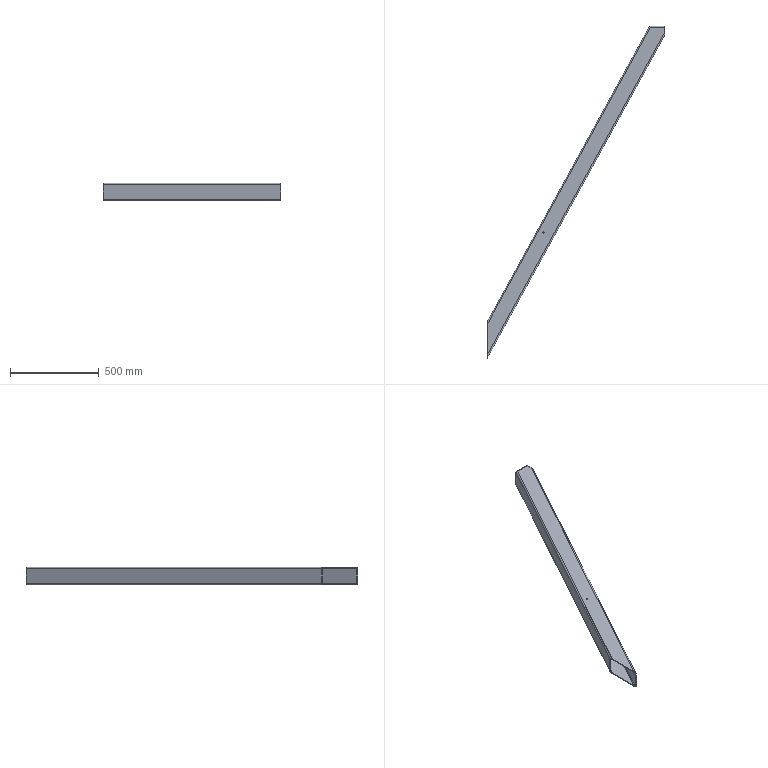Part | SolidWorks | features Fillet 2, Extrusion 1, HoleWzd 1, Shell 1 | 1 solid | 26 faces | box 1000 x 1874 x 100 mm | volume 3026106 mm3 | cylinder 14 | plane 12 | commonest cylinder face diameters 8.4 x6 16.4 x6 6.8 x2
STEP:
#1=CARTESIAN_POINT('',(312.6,708.43,96.));
#2=VERTEX_POINT('',#1);
#3=CARTESIAN_POINT('',(319.4,708.43,96.));
#4=VERTEX_POINT('',#3);
#5=CARTESIAN_POINT('',(316.,708.43,96.));
#6=DIRECTION('',(0.,0.,1.));
#7=DIRECTION('',(1.,0.,0.));
#8=AXIS2_PLACEMENT_3D('',#5,#6,#7);
#9=CIRCLE('',#8,3.4);
#10=EDGE_CURVE('',#2,#4,#9,.T.);
#11=ORIENTED_EDGE('',*,*,#10,.F.);
#12=CARTESIAN_POINT('',(312.6,708.43,100.));
#13=VERTEX_POINT('',#12);
#14=CARTESIAN_POINT('',(312.6,708.43,100.));
#15=DIRECTION('',(0.,0.,1.));
#16=VECTOR('',#15,1000.);
#17=LINE('',#14,#16);
#18=EDGE_CURVE('',#2,#13,#17,.T.);
#19=ORIENTED_EDGE('',*,*,#18,.T.);
#20=CARTESIAN_POINT('',(319.4,708.43,100.));
#21=VERTEX_POINT('',#20);
#22=CARTESIAN_POINT('',(316.,708.43,100.));
#23=DIRECTION('',(0.,0.,1.));
#24=DIRECTION('',(1.,0.,0.));
#25=AXIS2_PLACEMENT_3D('',#22,#23,#24);
#26=CIRCLE('',#25,3.4);
#27=EDGE_CURVE('',#13,#21,#26,.T.);
#28=ORIENTED_EDGE('',*,*,#27,.T.);
#29=CARTESIAN_POINT('',(319.4,708.43,100.));
#30=DIRECTION('',(0.,0.,1.));
#31=VECTOR('',#30,1000.);
#32=LINE('',#29,#31);
#33=EDGE_CURVE('',#4,#21,#32,.T.);
#34=ORIENTED_EDGE('',*,*,#33,.F.);
#35=EDGE_LOOP('',(#11,#19,#28,#34));
#36=FACE_OUTER_BOUND('',#35,.T.);
#37=CARTESIAN_POINT('',(316.,708.43,100.));
#38=DIRECTION('',(0.,0.,1.));
#39=DIRECTION('',(1.,0.,0.));
#40=AXIS2_PLACEMENT_3D('',#37,#38,#39);
#41=CYLINDRICAL_SURFACE('',#40,3.4);
#42=ADVANCED_FACE('',(#36),#41,.F.);
#43=CARTESIAN_POINT('',(1000.,1820.433,91.8));
#44=VERTEX_POINT('',#43);
#45=CARTESIAN_POINT('',(1000.,1820.433,8.2));
#46=VERTEX_POINT('',#45);
#47=CARTESIAN_POINT('',(1000.,1820.433,100.));
#48=DIRECTION('',(0.,0.,-1.));
#49=VECTOR('',#48,1000.);
#50=LINE('',#47,#49);
#51=EDGE_CURVE('',#44,#46,#50,.T.);
#52=ORIENTED_EDGE('',*,*,#51,.T.);
#53=CARTESIAN_POINT('',(1000.,1837.465,0.));
#54=VERTEX_POINT('',#53);
#55=CARTESIAN_POINT('',(1000.,1820.433,8.2));
#56=CARTESIAN_POINT('',(1000.,1820.433,3.397));
#57=CARTESIAN_POINT('',(1000.,1827.488,0.));
#58=CARTESIAN_POINT('',(1000.,1837.465,0.));
#59=(BOUNDED_CURVE()B_SPLINE_CURVE(3,(#55,#56,#57,#58),.UNSPECIFIED.,.F.,.F.)B_SPLINE_CURVE_WITH_KNOTS((4,4),(3.142,4.712),.UNSPECIFIED.)CURVE()GEOMETRIC_REPRESENTATION_ITEM()RATIONAL_B_SPLINE_CURVE((1.,0.8047,0.8047,1.))REPRESENTATION_ITEM(''));
#60=EDGE_CURVE('',#46,#54,#59,.T.);
#61=ORIENTED_EDGE('',*,*,#60,.T.);
#62=CARTESIAN_POINT('',(1000.,1866.233,0.));
#63=VERTEX_POINT('',#62);
#64=CARTESIAN_POINT('',(1000.,1874.433,0.));
#65=DIRECTION('',(0.,-1.,0.));
#66=VECTOR('',#65,1000.);
#67=LINE('',#64,#66);
#68=EDGE_CURVE('',#63,#54,#67,.T.);
#69=ORIENTED_EDGE('',*,*,#68,.F.);
#70=CARTESIAN_POINT('',(1000.,1874.433,8.2));
#71=VERTEX_POINT('',#70);
#72=CARTESIAN_POINT('',(1000.,1866.233,8.2));
#73=DIRECTION('',(1.,0.,0.));
#74=DIRECTION('',(0.,1.,0.));
#75=AXIS2_PLACEMENT_3D('',#72,#73,#74);
#76=CIRCLE('',#75,8.2);
#77=EDGE_CURVE('',#63,#71,#76,.T.);
#78=ORIENTED_EDGE('',*,*,#77,.T.);
#79=CARTESIAN_POINT('',(1000.,1874.433,91.8));
#80=VERTEX_POINT('',#79);
#81=CARTESIAN_POINT('',(1000.,1874.433,100.));
#82=DIRECTION('',(0.,0.,-1.));
#83=VECTOR('',#82,1000.);
#84=LINE('',#81,#83);
#85=EDGE_CURVE('',#80,#71,#84,.T.);
#86=ORIENTED_EDGE('',*,*,#85,.F.);
#87=CARTESIAN_POINT('',(1000.,1866.233,100.));
#88=VERTEX_POINT('',#87);
#89=CARTESIAN_POINT('',(1000.,1866.233,91.8));
#90=DIRECTION('',(1.,0.,0.));
#91=DIRECTION('',(0.,1.,0.));
#92=AXIS2_PLACEMENT_3D('',#89,#90,#91);
#93=CIRCLE('',#92,8.2);
#94=EDGE_CURVE('',#80,#88,#93,.T.);
#95=ORIENTED_EDGE('',*,*,#94,.T.);
#96=CARTESIAN_POINT('',(1000.,1837.465,100.));
#97=VERTEX_POINT('',#96);
#98=CARTESIAN_POINT('',(1000.,1874.433,100.));
#99=DIRECTION('',(0.,-1.,0.));
#100=VECTOR('',#99,1000.);
#101=LINE('',#98,#100);
#102=EDGE_CURVE('',#88,#97,#101,.T.);
#103=ORIENTED_EDGE('',*,*,#102,.T.);
#104=CARTESIAN_POINT('',(1000.,1837.465,100.));
#105=CARTESIAN_POINT('',(1000.,1827.488,100.));
#106=CARTESIAN_POINT('',(1000.,1820.433,96.603));
#107=CARTESIAN_POINT('',(1000.,1820.433,91.8));
#108=(BOUNDED_CURVE()B_SPLINE_CURVE(3,(#104,#105,#106,#107),.UNSPECIFIED.,.F.,.F.)B_SPLINE_CURVE_WITH_KNOTS((4,4),(4.712,6.283),.UNSPECIFIED.)CURVE()GEOMETRIC_REPRESENTATION_ITEM()RATIONAL_B_SPLINE_CURVE((1.,0.8047,0.8047,1.))REPRESENTATION_ITEM(''));
#109=EDGE_CURVE('',#97,#44,#108,.T.);
#110=ORIENTED_EDGE('',*,*,#109,.T.);
#111=EDGE_LOOP('',(#52,#61,#69,#78,#86,#95,#103,#110));
#112=FACE_OUTER_BOUND('',#111,.T.);
#113=CARTESIAN_POINT('',(1000.,1866.233,96.));
#114=VERTEX_POINT('',#113);
#115=CARTESIAN_POINT('',(1000.,1837.465,96.));
#116=VERTEX_POINT('',#115);
#117=CARTESIAN_POINT('',(1000.,1874.433,96.));
#118=DIRECTION('',(0.,-1.,0.));
#119=VECTOR('',#118,1000.);
#120=LINE('',#117,#119);
#121=EDGE_CURVE('',#114,#116,#120,.T.);
#122=ORIENTED_EDGE('',*,*,#121,.F.);
#123=CARTESIAN_POINT('',(1000.,1870.433,91.8));
#124=VERTEX_POINT('',#123);
#125=CARTESIAN_POINT('',(1000.,1866.233,91.8));
#126=DIRECTION('',(-1.,0.,0.));
#127=DIRECTION('',(0.,1.,0.));
#128=AXIS2_PLACEMENT_3D('',#125,#126,#127);
#129=CIRCLE('',#128,4.2);
#130=EDGE_CURVE('',#114,#124,#129,.T.);
#131=ORIENTED_EDGE('',*,*,#130,.T.);
#132=CARTESIAN_POINT('',(1000.,1870.433,8.2));
#133=VERTEX_POINT('',#132);
#134=CARTESIAN_POINT('',(1000.,1870.433,100.));
#135=DIRECTION('',(0.,0.,-1.));
#136=VECTOR('',#135,1000.);
#137=LINE('',#134,#136);
#138=EDGE_CURVE('',#124,#133,#137,.T.);
#139=ORIENTED_EDGE('',*,*,#138,.T.);
#140=CARTESIAN_POINT('',(1000.,1866.233,4.));
#141=VERTEX_POINT('',#140);
#142=CARTESIAN_POINT('',(1000.,1866.233,8.2));
#143=DIRECTION('',(-1.,0.,0.));
#144=DIRECTION('',(0.,1.,0.));
#145=AXIS2_PLACEMENT_3D('',#142,#143,#144);
#146=CIRCLE('',#145,4.2);
#147=EDGE_CURVE('',#133,#141,#146,.T.);
#148=ORIENTED_EDGE('',*,*,#147,.T.);
#149=CARTESIAN_POINT('',(1000.,1837.465,4.));
#150=VERTEX_POINT('',#149);
#151=CARTESIAN_POINT('',(1000.,1874.433,4.));
#152=DIRECTION('',(0.,-1.,0.));
#153=VECTOR('',#152,1000.);
#154=LINE('',#151,#153);
#155=EDGE_CURVE('',#141,#150,#154,.T.);
#156=ORIENTED_EDGE('',*,*,#155,.T.);
#157=CARTESIAN_POINT('',(1000.,1828.741,8.2));
#158=VERTEX_POINT('',#157);
#159=CARTESIAN_POINT('',(1000.,1837.465,4.));
#160=CARTESIAN_POINT('',(1000.,1832.355,4.));
#161=CARTESIAN_POINT('',(1000.,1828.741,5.74));
#162=CARTESIAN_POINT('',(1000.,1828.741,8.2));
#163=(BOUNDED_CURVE()B_SPLINE_CURVE(3,(#159,#160,#161,#162),.UNSPECIFIED.,.F.,.F.)B_SPLINE_CURVE_WITH_KNOTS((4,4),(4.712,6.283),.UNSPECIFIED.)CURVE()GEOMETRIC_REPRESENTATION_ITEM()RATIONAL_B_SPLINE_CURVE((1.,0.8047,0.8047,1.))REPRESENTATION_ITEM(''));
#164=EDGE_CURVE('',#150,#158,#163,.T.);
#165=ORIENTED_EDGE('',*,*,#164,.T.);
#166=CARTESIAN_POINT('',(1000.,1828.741,91.8));
#167=VERTEX_POINT('',#166);
#168=CARTESIAN_POINT('',(1000.,1828.741,100.));
#169=DIRECTION('',(0.,0.,-1.));
#170=VECTOR('',#169,1000.);
#171=LINE('',#168,#170);
#172=EDGE_CURVE('',#167,#158,#171,.T.);
#173=ORIENTED_EDGE('',*,*,#172,.F.);
#174=CARTESIAN_POINT('',(1000.,1828.741,91.8));
#175=CARTESIAN_POINT('',(1000.,1828.741,94.26));
#176=CARTESIAN_POINT('',(1000.,1832.355,96.));
#177=CARTESIAN_POINT('',(1000.,1837.465,96.));
#178=(BOUNDED_CURVE()B_SPLINE_CURVE(3,(#174,#175,#176,#177),.UNSPECIFIED.,.F.,.F.)B_SPLINE_CURVE_WITH_KNOTS((4,4),(3.142,4.712),.UNSPECIFIED.)CURVE()GEOMETRIC_REPRESENTATION_ITEM()RATIONAL_B_SPLINE_CURVE((1.,0.8047,0.8047,1.))REPRESENTATION_ITEM(''));
#179=EDGE_CURVE('',#167,#116,#178,.T.);
#180=ORIENTED_EDGE('',*,*,#179,.T.);
#181=EDGE_LOOP('',(#122,#131,#139,#148,#156,#165,#173,#180));
#182=FACE_BOUND('',#181,.T.);
#183=CARTESIAN_POINT('',(1000.,1874.433,100.));
#184=DIRECTION('',(1.,0.,0.));
#185=DIRECTION('',(0.,1.,0.));
#186=AXIS2_PLACEMENT_3D('',#183,#184,#185);
#187=PLANE('',#186);
#188=ADVANCED_FACE('',(#112,#182),#187,.T.);
#189=CARTESIAN_POINT('',(0.,17.031,0.));
#190=VERTEX_POINT('',#189);
#191=CARTESIAN_POINT('',(0.,191.705,0.));
#192=VERTEX_POINT('',#191);
#193=CARTESIAN_POINT('',(0.,0.,0.));
#194=DIRECTION('',(0.,1.,0.));
#195=VECTOR('',#194,1000.);
#196=LINE('',#193,#195);
#197=EDGE_CURVE('',#190,#192,#196,.T.);
#198=ORIENTED_EDGE('',*,*,#197,.F.);
#199=CARTESIAN_POINT('',(0.,0.,8.2));
#200=VERTEX_POINT('',#199);
#201=CARTESIAN_POINT('',(0.,17.031,0.));
#202=CARTESIAN_POINT('',(0.,7.055,0.));
#203=CARTESIAN_POINT('',(0.,0.,3.397));
#204=CARTESIAN_POINT('',(0.,0.,8.2));
#205=(BOUNDED_CURVE()B_SPLINE_CURVE(3,(#201,#202,#203,#204),.UNSPECIFIED.,.F.,.F.)B_SPLINE_CURVE_WITH_KNOTS((4,4),(1.571,3.142),.UNSPECIFIED.)CURVE()GEOMETRIC_REPRESENTATION_ITEM()RATIONAL_B_SPLINE_CURVE((1.,0.8047,0.8047,1.))REPRESENTATION_ITEM(''));
#206=EDGE_CURVE('',#190,#200,#205,.T.);
#207=ORIENTED_EDGE('',*,*,#206,.T.);
#208=CARTESIAN_POINT('',(0.,0.,91.8));
#209=VERTEX_POINT('',#208);
#210=CARTESIAN_POINT('',(0.,0.,100.));
#211=DIRECTION('',(0.,0.,-1.));
#212=VECTOR('',#211,1000.);
#213=LINE('',#210,#212);
#214=EDGE_CURVE('',#209,#200,#213,.T.);
#215=ORIENTED_EDGE('',*,*,#214,.F.);
#216=CARTESIAN_POINT('',(0.,17.031,100.));
#217=VERTEX_POINT('',#216);
#218=CARTESIAN_POINT('',(0.,0.,91.8));
#219=CARTESIAN_POINT('',(0.,0.,96.603));
#220=CARTESIAN_POINT('',(0.,7.055,100.));
#221=CARTESIAN_POINT('',(0.,17.031,100.));
#222=(BOUNDED_CURVE()B_SPLINE_CURVE(3,(#218,#219,#220,#221),.UNSPECIFIED.,.F.,.F.)B_SPLINE_CURVE_WITH_KNOTS((4,4),(0.,1.571),.UNSPECIFIED.)CURVE()GEOMETRIC_REPRESENTATION_ITEM()RATIONAL_B_SPLINE_CURVE((1.,0.8047,0.8047,1.))REPRESENTATION_ITEM(''));
#223=EDGE_CURVE('',#209,#217,#222,.T.);
#224=ORIENTED_EDGE('',*,*,#223,.T.);
#225=CARTESIAN_POINT('',(0.,191.705,100.));
#226=VERTEX_POINT('',#225);
#227=CARTESIAN_POINT('',(0.,0.,100.));
#228=DIRECTION('',(0.,1.,0.));
#229=VECTOR('',#228,1000.);
#230=LINE('',#227,#229);
#231=EDGE_CURVE('',#217,#226,#230,.T.);
#232=ORIENTED_EDGE('',*,*,#231,.T.);
#233=CARTESIAN_POINT('',(0.,208.737,91.8));
#234=VERTEX_POINT('',#233);
#235=CARTESIAN_POINT('',(0.,191.705,100.));
#236=CARTESIAN_POINT('',(0.,201.682,100.));
#237=CARTESIAN_POINT('',(0.,208.737,96.603));
#238=CARTESIAN_POINT('',(0.,208.737,91.8));
#239=(BOUNDED_CURVE()B_SPLINE_CURVE(3,(#235,#236,#237,#238),.UNSPECIFIED.,.F.,.T.)B_SPLINE_CURVE_WITH_KNOTS((4,4),(4.712,6.283),.UNSPECIFIED.)CURVE()GEOMETRIC_REPRESENTATION_ITEM()RATIONAL_B_SPLINE_CURVE((1.,0.8047,0.8047,1.))REPRESENTATION_ITEM(''));
#240=EDGE_CURVE('',#226,#234,#239,.T.);
#241=ORIENTED_EDGE('',*,*,#240,.T.);
#242=CARTESIAN_POINT('',(0.,208.737,8.2));
#243=VERTEX_POINT('',#242);
#244=CARTESIAN_POINT('',(0.,208.737,100.));
#245=DIRECTION('',(0.,0.,-1.));
#246=VECTOR('',#245,1000.);
#247=LINE('',#244,#246);
#248=EDGE_CURVE('',#234,#243,#247,.T.);
#249=ORIENTED_EDGE('',*,*,#248,.T.);
#250=CARTESIAN_POINT('',(0.,208.737,8.2));
#251=CARTESIAN_POINT('',(0.,208.737,3.397));
#252=CARTESIAN_POINT('',(0.,201.682,0.));
#253=CARTESIAN_POINT('',(0.,191.705,0.));
#254=(BOUNDED_CURVE()B_SPLINE_CURVE(3,(#250,#251,#252,#253),.UNSPECIFIED.,.F.,.F.)B_SPLINE_CURVE_WITH_KNOTS((4,4),(3.142,4.712),.UNSPECIFIED.)CURVE()GEOMETRIC_REPRESENTATION_ITEM()RATIONAL_B_SPLINE_CURVE((1.,0.8047,0.8047,1.))REPRESENTATION_ITEM(''));
#255=EDGE_CURVE('',#243,#192,#254,.T.);
#256=ORIENTED_EDGE('',*,*,#255,.T.);
#257=EDGE_LOOP('',(#198,#207,#215,#224,#232,#241,#249,#256));
#258=FACE_OUTER_BOUND('',#257,.T.);
#259=CARTESIAN_POINT('',(0.,17.031,96.));
#260=VERTEX_POINT('',#259);
#261=CARTESIAN_POINT('',(0.,191.705,96.));
#262=VERTEX_POINT('',#261);
#263=CARTESIAN_POINT('',(0.,0.,96.));
#264=DIRECTION('',(0.,1.,0.));
#265=VECTOR('',#264,1000.);
#266=LINE('',#263,#265);
#267=EDGE_CURVE('',#260,#262,#266,.T.);
#268=ORIENTED_EDGE('',*,*,#267,.F.);
#269=CARTESIAN_POINT('',(0.,8.308,91.8));
#270=VERTEX_POINT('',#269);
#271=CARTESIAN_POINT('',(0.,17.031,96.));
#272=CARTESIAN_POINT('',(0.,11.921,96.));
#273=CARTESIAN_POINT('',(0.,8.308,94.26));
#274=CARTESIAN_POINT('',(0.,8.308,91.8));
#275=(BOUNDED_CURVE()B_SPLINE_CURVE(3,(#271,#272,#273,#274),.UNSPECIFIED.,.F.,.F.)B_SPLINE_CURVE_WITH_KNOTS((4,4),(1.571,3.142),.UNSPECIFIED.)CURVE()GEOMETRIC_REPRESENTATION_ITEM()RATIONAL_B_SPLINE_CURVE((1.,0.8047,0.8047,1.))REPRESENTATION_ITEM(''));
#276=EDGE_CURVE('',#260,#270,#275,.T.);
#277=ORIENTED_EDGE('',*,*,#276,.T.);
#278=CARTESIAN_POINT('',(0.,8.308,8.2));
#279=VERTEX_POINT('',#278);
#280=CARTESIAN_POINT('',(0.,8.308,100.));
#281=DIRECTION('',(0.,0.,-1.));
#282=VECTOR('',#281,1000.);
#283=LINE('',#280,#282);
#284=EDGE_CURVE('',#270,#279,#283,.T.);
#285=ORIENTED_EDGE('',*,*,#284,.T.);
#286=CARTESIAN_POINT('',(0.,17.031,4.));
#287=VERTEX_POINT('',#286);
#288=CARTESIAN_POINT('',(0.,8.308,8.2));
#289=CARTESIAN_POINT('',(0.,8.308,5.74));
#290=CARTESIAN_POINT('',(0.,11.921,4.));
#291=CARTESIAN_POINT('',(0.,17.031,4.));
#292=(BOUNDED_CURVE()B_SPLINE_CURVE(3,(#288,#289,#290,#291),.UNSPECIFIED.,.F.,.F.)B_SPLINE_CURVE_WITH_KNOTS((4,4),(0.,1.571),.UNSPECIFIED.)CURVE()GEOMETRIC_REPRESENTATION_ITEM()RATIONAL_B_SPLINE_CURVE((1.,0.8047,0.8047,1.))REPRESENTATION_ITEM(''));
#293=EDGE_CURVE('',#279,#287,#292,.T.);
#294=ORIENTED_EDGE('',*,*,#293,.T.);
#295=CARTESIAN_POINT('',(0.,191.705,4.));
#296=VERTEX_POINT('',#295);
#297=CARTESIAN_POINT('',(0.,0.,4.));
#298=DIRECTION('',(0.,1.,0.));
#299=VECTOR('',#298,1000.);
#300=LINE('',#297,#299);
#301=EDGE_CURVE('',#287,#296,#300,.T.);
#302=ORIENTED_EDGE('',*,*,#301,.T.);
#303=CARTESIAN_POINT('',(0.,200.429,8.2));
#304=VERTEX_POINT('',#303);
#305=CARTESIAN_POINT('',(0.,191.705,4.));
#306=CARTESIAN_POINT('',(0.,196.815,4.));
#307=CARTESIAN_POINT('',(0.,200.429,5.74));
#308=CARTESIAN_POINT('',(0.,200.429,8.2));
#309=(BOUNDED_CURVE()B_SPLINE_CURVE(3,(#305,#306,#307,#308),.UNSPECIFIED.,.F.,.F.)B_SPLINE_CURVE_WITH_KNOTS((4,4),(4.712,6.283),.UNSPECIFIED.)CURVE()GEOMETRIC_REPRESENTATION_ITEM()RATIONAL_B_SPLINE_CURVE((1.,0.8047,0.8047,1.))REPRESENTATION_ITEM(''));
#310=EDGE_CURVE('',#296,#304,#309,.T.);
#311=ORIENTED_EDGE('',*,*,#310,.T.);
#312=CARTESIAN_POINT('',(0.,200.429,91.8));
#313=VERTEX_POINT('',#312);
#314=CARTESIAN_POINT('',(0.,200.429,100.));
#315=DIRECTION('',(0.,0.,-1.));
#316=VECTOR('',#315,1000.);
#317=LINE('',#314,#316);
#318=EDGE_CURVE('',#313,#304,#317,.T.);
#319=ORIENTED_EDGE('',*,*,#318,.F.);
#320=CARTESIAN_POINT('',(0.,200.429,91.8));
#321=CARTESIAN_POINT('',(0.,200.429,94.26));
#322=CARTESIAN_POINT('',(0.,196.815,96.));
#323=CARTESIAN_POINT('',(0.,191.705,96.));
#324=(BOUNDED_CURVE()B_SPLINE_CURVE(3,(#320,#321,#322,#323),.UNSPECIFIED.,.F.,.T.)B_SPLINE_CURVE_WITH_KNOTS((4,4),(3.142,4.712),.UNSPECIFIED.)CURVE()GEOMETRIC_REPRESENTATION_ITEM()RATIONAL_B_SPLINE_CURVE((1.,0.8047,0.8047,1.))REPRESENTATION_ITEM(''));
#325=EDGE_CURVE('',#313,#262,#324,.T.);
#326=ORIENTED_EDGE('',*,*,#325,.T.);
#327=EDGE_LOOP('',(#268,#277,#285,#294,#302,#311,#319,#326));
#328=FACE_BOUND('',#327,.T.);
#329=CARTESIAN_POINT('',(0.,0.,100.));
#330=DIRECTION('',(-1.,0.,0.));
#331=DIRECTION('',(0.,-1.,0.));
#332=AXIS2_PLACEMENT_3D('',#329,#330,#331);
#333=PLANE('',#332);
#334=ADVANCED_FACE('',(#258,#328),#333,.T.);
#335=ORIENTED_EDGE('',*,*,#85,.T.);
#336=CARTESIAN_POINT('',(915.,1874.433,8.2));
#337=VERTEX_POINT('',#336);
#338=CARTESIAN_POINT('',(915.,1874.433,8.2));
#339=DIRECTION('',(-1.,0.,0.));
#340=VECTOR('',#339,1000.);
#341=LINE('',#338,#340);
#342=EDGE_CURVE('',#71,#337,#341,.T.);
#343=ORIENTED_EDGE('',*,*,#342,.T.);
#344=CARTESIAN_POINT('',(915.,1874.433,91.8));
#345=VERTEX_POINT('',#344);
#346=CARTESIAN_POINT('',(915.,1874.433,100.));
#347=DIRECTION('',(0.,0.,-1.));
#348=VECTOR('',#347,1000.);
#349=LINE('',#346,#348);
#350=EDGE_CURVE('',#345,#337,#349,.T.);
#351=ORIENTED_EDGE('',*,*,#350,.F.);
#352=CARTESIAN_POINT('',(915.,1874.433,91.8));
#353=DIRECTION('',(1.,0.,0.));
#354=VECTOR('',#353,1000.);
#355=LINE('',#352,#354);
#356=EDGE_CURVE('',#345,#80,#355,.T.);
#357=ORIENTED_EDGE('',*,*,#356,.T.);
#358=EDGE_LOOP('',(#335,#343,#351,#357));
#359=FACE_OUTER_BOUND('',#358,.T.);
#360=CARTESIAN_POINT('',(915.,1874.433,100.));
#361=DIRECTION('',(0.,1.,0.));
#362=DIRECTION('',(-1.,0.,0.));
#363=AXIS2_PLACEMENT_3D('',#360,#361,#362);
#364=PLANE('',#363);
#365=ADVANCED_FACE('',(#359),#364,.T.);
#366=ORIENTED_EDGE('',*,*,#350,.T.);
#367=CARTESIAN_POINT('',(0.,208.737,8.2));
#368=DIRECTION('',(-0.4815,-0.8765,0.));
#369=VECTOR('',#368,1000.);
#370=LINE('',#367,#369);
#371=EDGE_CURVE('',#337,#243,#370,.T.);
#372=ORIENTED_EDGE('',*,*,#371,.T.);
#373=ORIENTED_EDGE('',*,*,#248,.F.);
#374=CARTESIAN_POINT('',(0.,208.737,91.8));
#375=DIRECTION('',(0.4815,0.8765,0.));
#376=VECTOR('',#375,1000.);
#377=LINE('',#374,#376);
#378=EDGE_CURVE('',#234,#345,#377,.T.);
#379=ORIENTED_EDGE('',*,*,#378,.T.);
#380=EDGE_LOOP('',(#366,#372,#373,#379));
#381=FACE_OUTER_BOUND('',#380,.T.);
#382=CARTESIAN_POINT('',(0.,208.737,100.));
#383=DIRECTION('',(-0.8765,0.4815,0.));
#384=DIRECTION('',(-0.4815,-0.8765,0.));
#385=AXIS2_PLACEMENT_3D('',#382,#383,#384);
#386=PLANE('',#385);
#387=ADVANCED_FACE('',(#381),#386,.T.);
#388=ORIENTED_EDGE('',*,*,#214,.T.);
#389=CARTESIAN_POINT('',(1000.,1820.433,8.2));
#390=DIRECTION('',(0.4815,0.8765,0.));
#391=VECTOR('',#390,1000.);
#392=LINE('',#389,#391);
#393=EDGE_CURVE('',#200,#46,#392,.T.);
#394=ORIENTED_EDGE('',*,*,#393,.T.);
#395=ORIENTED_EDGE('',*,*,#51,.F.);
#396=CARTESIAN_POINT('',(1000.,1820.433,91.8));
#397=DIRECTION('',(-0.4815,-0.8765,0.));
#398=VECTOR('',#397,1000.);
#399=LINE('',#396,#398);
#400=EDGE_CURVE('',#44,#209,#399,.T.);
#401=ORIENTED_EDGE('',*,*,#400,.T.);
#402=EDGE_LOOP('',(#388,#394,#395,#401));
#403=FACE_OUTER_BOUND('',#402,.T.);
#404=CARTESIAN_POINT('',(1000.,1820.433,100.));
#405=DIRECTION('',(0.8765,-0.4815,0.));
#406=DIRECTION('',(0.4815,0.8765,0.));
#407=AXIS2_PLACEMENT_3D('',#404,#405,#406);
#408=PLANE('',#407);
#409=ADVANCED_FACE('',(#403),#408,.T.);
#410=CARTESIAN_POINT('',(316.,708.43,100.));
#411=DIRECTION('',(0.,0.,1.));
#412=DIRECTION('',(1.,0.,0.));
#413=AXIS2_PLACEMENT_3D('',#410,#411,#412);
#414=CIRCLE('',#413,3.4);
#415=EDGE_CURVE('',#21,#13,#414,.T.);
#416=ORIENTED_EDGE('',*,*,#415,.F.);
#417=ORIENTED_EDGE('',*,*,#27,.F.);
#418=EDGE_LOOP('',(#416,#417));
#419=FACE_BOUND('',#418,.T.);
#420=ORIENTED_EDGE('',*,*,#231,.F.);
#421=CARTESIAN_POINT('',(-7.187,3.948,100.));
#422=DIRECTION('',(0.4815,0.8765,0.));
#423=VECTOR('',#422,1000.);
#424=LINE('',#421,#423);
#425=EDGE_CURVE('',#217,#97,#424,.T.);
#426=ORIENTED_EDGE('',*,*,#425,.T.);
#427=ORIENTED_EDGE('',*,*,#102,.F.);
#428=CARTESIAN_POINT('',(919.851,1866.233,100.));
#429=VERTEX_POINT('',#428);
#430=CARTESIAN_POINT('',(0.,1866.233,100.));
#431=DIRECTION('',(-1.,0.,0.));
#432=VECTOR('',#431,1000.);
#433=LINE('',#430,#432);
#434=EDGE_CURVE('',#88,#429,#433,.T.);
#435=ORIENTED_EDGE('',*,*,#434,.T.);
#436=CARTESIAN_POINT('',(-80.897,44.438,100.));
#437=DIRECTION('',(-0.4815,-0.8765,0.));
#438=VECTOR('',#437,1000.);
#439=LINE('',#436,#438);
#440=EDGE_CURVE('',#429,#226,#439,.T.);
#441=ORIENTED_EDGE('',*,*,#440,.T.);
#442=EDGE_LOOP('',(#420,#426,#427,#435,#441));
#443=FACE_OUTER_BOUND('',#442,.T.);
#444=CARTESIAN_POINT('',(0.,0.,100.));
#445=DIRECTION('',(0.,0.,1.));
#446=DIRECTION('',(1.,0.,0.));
#447=AXIS2_PLACEMENT_3D('',#444,#445,#446);
#448=PLANE('',#447);
#449=ADVANCED_FACE('',(#419,#443),#448,.T.);
#450=ORIENTED_EDGE('',*,*,#68,.T.);
#451=CARTESIAN_POINT('',(-7.187,3.948,0.));
#452=DIRECTION('',(-0.4815,-0.8765,0.));
#453=VECTOR('',#452,1000.);
#454=LINE('',#451,#453);
#455=EDGE_CURVE('',#54,#190,#454,.T.);
#456=ORIENTED_EDGE('',*,*,#455,.T.);
#457=ORIENTED_EDGE('',*,*,#197,.T.);
#458=CARTESIAN_POINT('',(919.851,1866.233,0.));
#459=VERTEX_POINT('',#458);
#460=CARTESIAN_POINT('',(922.187,1870.485,0.));
#461=DIRECTION('',(0.4815,0.8765,0.));
#462=VECTOR('',#461,1000.);
#463=LINE('',#460,#462);
#464=EDGE_CURVE('',#192,#459,#463,.T.);
#465=ORIENTED_EDGE('',*,*,#464,.T.);
#466=CARTESIAN_POINT('',(1000.,1866.233,0.));
#467=DIRECTION('',(1.,0.,0.));
#468=VECTOR('',#467,1000.);
#469=LINE('',#466,#468);
#470=EDGE_CURVE('',#459,#63,#469,.T.);
#471=ORIENTED_EDGE('',*,*,#470,.T.);
#472=EDGE_LOOP('',(#450,#456,#457,#465,#471));
#473=FACE_OUTER_BOUND('',#472,.T.);
#474=CARTESIAN_POINT('',(0.,0.,0.));
#475=DIRECTION('',(0.,0.,1.));
#476=DIRECTION('',(1.,0.,0.));
#477=AXIS2_PLACEMENT_3D('',#474,#475,#476);
#478=PLANE('',#477);
#479=ADVANCED_FACE('',(#473),#478,.F.);
#480=ORIENTED_EDGE('',*,*,#138,.F.);
#481=CARTESIAN_POINT('',(917.366,1870.433,91.8));
#482=VERTEX_POINT('',#481);
#483=CARTESIAN_POINT('',(917.366,1870.433,91.8));
#484=DIRECTION('',(-1.,0.,0.));
#485=VECTOR('',#484,1000.);
#486=LINE('',#483,#485);
#487=EDGE_CURVE('',#124,#482,#486,.T.);
#488=ORIENTED_EDGE('',*,*,#487,.T.);
#489=CARTESIAN_POINT('',(917.366,1870.433,8.2));
#490=VERTEX_POINT('',#489);
#491=CARTESIAN_POINT('',(917.366,1870.433,100.));
#492=DIRECTION('',(0.,0.,-1.));
#493=VECTOR('',#492,1000.);
#494=LINE('',#491,#493);
#495=EDGE_CURVE('',#482,#490,#494,.T.);
#496=ORIENTED_EDGE('',*,*,#495,.T.);
#497=CARTESIAN_POINT('',(915.,1870.433,8.2));
#498=DIRECTION('',(1.,0.,0.));
#499=VECTOR('',#498,1000.);
#500=LINE('',#497,#499);
#501=EDGE_CURVE('',#490,#133,#500,.T.);
#502=ORIENTED_EDGE('',*,*,#501,.T.);
#503=EDGE_LOOP('',(#480,#488,#496,#502));
#504=FACE_OUTER_BOUND('',#503,.T.);
#505=CARTESIAN_POINT('',(915.,1870.433,100.));
#506=DIRECTION('',(0.,1.,0.));
#507=DIRECTION('',(-1.,0.,0.));
#508=AXIS2_PLACEMENT_3D('',#505,#506,#507);
#509=PLANE('',#508);
#510=ADVANCED_FACE('',(#504),#509,.F.);
#511=ORIENTED_EDGE('',*,*,#318,.T.);
#512=CARTESIAN_POINT('',(3.506,206.811,8.2));
#513=DIRECTION('',(0.4815,0.8765,0.));
#514=VECTOR('',#513,1000.);
#515=LINE('',#512,#514);
#516=EDGE_CURVE('',#304,#490,#515,.T.);
#517=ORIENTED_EDGE('',*,*,#516,.T.);
#518=ORIENTED_EDGE('',*,*,#495,.F.);
#519=CARTESIAN_POINT('',(0.,200.429,91.8));
#520=DIRECTION('',(-0.4815,-0.8765,0.));
#521=VECTOR('',#520,1000.);
#522=LINE('',#519,#521);
#523=EDGE_CURVE('',#482,#313,#522,.T.);
#524=ORIENTED_EDGE('',*,*,#523,.T.);
#525=EDGE_LOOP('',(#511,#517,#518,#524));
#526=FACE_OUTER_BOUND('',#525,.T.);
#527=CARTESIAN_POINT('',(3.506,206.811,100.));
#528=DIRECTION('',(-0.8765,0.4815,0.));
#529=DIRECTION('',(-0.4815,-0.8765,0.));
#530=AXIS2_PLACEMENT_3D('',#527,#528,#529);
#531=PLANE('',#530);
#532=ADVANCED_FACE('',(#526),#531,.F.);
#533=ORIENTED_EDGE('',*,*,#284,.F.);
#534=CARTESIAN_POINT('',(1000.,1828.741,91.8));
#535=DIRECTION('',(0.4815,0.8765,0.));
#536=VECTOR('',#535,1000.);
#537=LINE('',#534,#536);
#538=EDGE_CURVE('',#270,#167,#537,.T.);
#539=ORIENTED_EDGE('',*,*,#538,.T.);
#540=ORIENTED_EDGE('',*,*,#172,.T.);
#541=CARTESIAN_POINT('',(996.494,1822.359,8.2));
#542=DIRECTION('',(-0.4815,-0.8765,0.));
#543=VECTOR('',#542,1000.);
#544=LINE('',#541,#543);
#545=EDGE_CURVE('',#158,#279,#544,.T.);
#546=ORIENTED_EDGE('',*,*,#545,.T.);
#547=EDGE_LOOP('',(#533,#539,#540,#546));
#548=FACE_OUTER_BOUND('',#547,.T.);
#549=CARTESIAN_POINT('',(996.494,1822.359,100.));
#550=DIRECTION('',(0.8765,-0.4815,0.));
#551=DIRECTION('',(0.4815,0.8765,0.));
#552=AXIS2_PLACEMENT_3D('',#549,#550,#551);
#553=PLANE('',#552);
#554=ADVANCED_FACE('',(#548),#553,.F.);
#555=CARTESIAN_POINT('',(316.,708.43,96.));
#556=DIRECTION('',(0.,0.,1.));
#557=DIRECTION('',(1.,0.,0.));
#558=AXIS2_PLACEMENT_3D('',#555,#556,#557);
#559=CIRCLE('',#558,3.4);
#560=EDGE_CURVE('',#4,#2,#559,.T.);
#561=ORIENTED_EDGE('',*,*,#560,.T.);
#562=ORIENTED_EDGE('',*,*,#10,.T.);
#563=EDGE_LOOP('',(#561,#562));
#564=FACE_BOUND('',#563,.T.);
#565=ORIENTED_EDGE('',*,*,#121,.T.);
#566=CARTESIAN_POINT('',(-3.681,10.33,96.));
#567=DIRECTION('',(-0.4815,-0.8765,0.));
#568=VECTOR('',#567,1000.);
#569=LINE('',#566,#568);
#570=EDGE_CURVE('',#116,#260,#569,.T.);
#571=ORIENTED_EDGE('',*,*,#570,.T.);
#572=ORIENTED_EDGE('',*,*,#267,.T.);
#573=CARTESIAN_POINT('',(919.851,1866.233,96.));
#574=VERTEX_POINT('',#573);
#575=CARTESIAN_POINT('',(921.048,1868.411,96.));
#576=DIRECTION('',(0.4815,0.8765,0.));
#577=VECTOR('',#576,1000.);
#578=LINE('',#575,#577);
#579=EDGE_CURVE('',#262,#574,#578,.T.);
#580=ORIENTED_EDGE('',*,*,#579,.T.);
#581=CARTESIAN_POINT('',(1000.,1866.233,96.));
#582=DIRECTION('',(1.,0.,0.));
#583=VECTOR('',#582,1000.);
#584=LINE('',#581,#583);
#585=EDGE_CURVE('',#574,#114,#584,.T.);
#586=ORIENTED_EDGE('',*,*,#585,.T.);
#587=EDGE_LOOP('',(#565,#571,#572,#580,#586));
#588=FACE_OUTER_BOUND('',#587,.T.);
#589=CARTESIAN_POINT('',(0.,0.,96.));
#590=DIRECTION('',(0.,0.,1.));
#591=DIRECTION('',(1.,0.,0.));
#592=AXIS2_PLACEMENT_3D('',#589,#590,#591);
#593=PLANE('',#592);
#594=ADVANCED_FACE('',(#564,#588),#593,.F.);
#595=ORIENTED_EDGE('',*,*,#301,.F.);
#596=CARTESIAN_POINT('',(-7.187,3.948,4.));
#597=DIRECTION('',(0.4815,0.8765,0.));
#598=VECTOR('',#597,1000.);
#599=LINE('',#596,#598);
#600=EDGE_CURVE('',#287,#150,#599,.T.);
#601=ORIENTED_EDGE('',*,*,#600,.T.);
#602=ORIENTED_EDGE('',*,*,#155,.F.);
#603=CARTESIAN_POINT('',(919.851,1866.233,4.));
#604=VERTEX_POINT('',#603);
#605=CARTESIAN_POINT('',(0.,1866.233,4.));
#606=DIRECTION('',(-1.,0.,0.));
#607=VECTOR('',#606,1000.);
#608=LINE('',#605,#607);
#609=EDGE_CURVE('',#141,#604,#608,.T.);
#610=ORIENTED_EDGE('',*,*,#609,.T.);
#611=CARTESIAN_POINT('',(-80.897,44.438,4.));
#612=DIRECTION('',(-0.4815,-0.8765,0.));
#613=VECTOR('',#612,1000.);
#614=LINE('',#611,#613);
#615=EDGE_CURVE('',#604,#296,#614,.T.);
#616=ORIENTED_EDGE('',*,*,#615,.T.);
#617=EDGE_LOOP('',(#595,#601,#602,#610,#616));
#618=FACE_OUTER_BOUND('',#617,.T.);
#619=CARTESIAN_POINT('',(0.,0.,4.));
#620=DIRECTION('',(0.,0.,1.));
#621=DIRECTION('',(1.,0.,0.));
#622=AXIS2_PLACEMENT_3D('',#619,#620,#621);
#623=PLANE('',#622);
#624=ADVANCED_FACE('',(#618),#623,.T.);
#625=ORIENTED_EDGE('',*,*,#60,.F.);
#626=ORIENTED_EDGE('',*,*,#393,.F.);
#627=ORIENTED_EDGE('',*,*,#206,.F.);
#628=ORIENTED_EDGE('',*,*,#455,.F.);
#629=EDGE_LOOP('',(#625,#626,#627,#628));
#630=FACE_OUTER_BOUND('',#629,.T.);
#631=CARTESIAN_POINT('',(-7.187,3.948,8.2));
#632=DIRECTION('',(0.4815,0.8765,0.));
#633=DIRECTION('',(-0.8765,0.4815,0.));
#634=AXIS2_PLACEMENT_3D('',#631,#632,#633);
#635=CYLINDRICAL_SURFACE('',#634,8.2);
#636=ADVANCED_FACE('',(#630),#635,.T.);
#637=ORIENTED_EDGE('',*,*,#77,.F.);
#638=ORIENTED_EDGE('',*,*,#470,.F.);
#639=CARTESIAN_POINT('',(915.,1874.433,8.2));
#640=CARTESIAN_POINT('',(915.,1874.433,3.397));
#641=CARTESIAN_POINT('',(917.009,1871.037,0.));
#642=CARTESIAN_POINT('',(919.851,1866.233,0.));
#643=(BOUNDED_CURVE()B_SPLINE_CURVE(3,(#639,#640,#641,#642),.UNSPECIFIED.,.F.,.F.)B_SPLINE_CURVE_WITH_KNOTS((4,4),(0.,1.571),.UNSPECIFIED.)CURVE()GEOMETRIC_REPRESENTATION_ITEM()RATIONAL_B_SPLINE_CURVE((1.,0.8047,0.8047,1.))REPRESENTATION_ITEM(''));
#644=EDGE_CURVE('',#337,#459,#643,.T.);
#645=ORIENTED_EDGE('',*,*,#644,.F.);
#646=ORIENTED_EDGE('',*,*,#342,.F.);
#647=EDGE_LOOP('',(#637,#638,#645,#646));
#648=FACE_OUTER_BOUND('',#647,.T.);
#649=CARTESIAN_POINT('',(0.,1866.233,8.2));
#650=DIRECTION('',(-1.,0.,0.));
#651=DIRECTION('',(0.,-1.,0.));
#652=AXIS2_PLACEMENT_3D('',#649,#650,#651);
#653=CYLINDRICAL_SURFACE('',#652,8.2);
#654=ADVANCED_FACE('',(#648),#653,.T.);
#655=ORIENTED_EDGE('',*,*,#255,.F.);
#656=ORIENTED_EDGE('',*,*,#371,.F.);
#657=ORIENTED_EDGE('',*,*,#644,.T.);
#658=ORIENTED_EDGE('',*,*,#464,.F.);
#659=EDGE_LOOP('',(#655,#656,#657,#658));
#660=FACE_OUTER_BOUND('',#659,.T.);
#661=CARTESIAN_POINT('',(-80.897,44.438,8.2));
#662=DIRECTION('',(-0.4815,-0.8765,0.));
#663=DIRECTION('',(0.8765,-0.4815,0.));
#664=AXIS2_PLACEMENT_3D('',#661,#662,#663);
#665=CYLINDRICAL_SURFACE('',#664,8.2);
#666=ADVANCED_FACE('',(#660),#665,.T.);
#667=ORIENTED_EDGE('',*,*,#240,.F.);
#668=ORIENTED_EDGE('',*,*,#440,.F.);
#669=CARTESIAN_POINT('',(915.,1874.433,91.8));
#670=CARTESIAN_POINT('',(915.,1874.433,96.603));
#671=CARTESIAN_POINT('',(917.009,1871.037,100.));
#672=CARTESIAN_POINT('',(919.851,1866.233,100.));
#673=(BOUNDED_CURVE()B_SPLINE_CURVE(3,(#669,#670,#671,#672),.UNSPECIFIED.,.F.,.T.)B_SPLINE_CURVE_WITH_KNOTS((4,4),(0.,1.571),.UNSPECIFIED.)CURVE()GEOMETRIC_REPRESENTATION_ITEM()RATIONAL_B_SPLINE_CURVE((1.,0.8047,0.8047,1.))REPRESENTATION_ITEM(''));
#674=EDGE_CURVE('',#345,#429,#673,.T.);
#675=ORIENTED_EDGE('',*,*,#674,.F.);
#676=ORIENTED_EDGE('',*,*,#378,.F.);
#677=EDGE_LOOP('',(#667,#668,#675,#676));
#678=FACE_OUTER_BOUND('',#677,.T.);
#679=CARTESIAN_POINT('',(7.187,204.789,91.8));
#680=DIRECTION('',(0.4815,0.8765,0.));
#681=DIRECTION('',(-0.8765,0.4815,0.));
#682=AXIS2_PLACEMENT_3D('',#679,#680,#681);
#683=CYLINDRICAL_SURFACE('',#682,8.2);
#684=ADVANCED_FACE('',(#678),#683,.T.);
#685=ORIENTED_EDGE('',*,*,#674,.T.);
#686=ORIENTED_EDGE('',*,*,#434,.F.);
#687=ORIENTED_EDGE('',*,*,#94,.F.);
#688=ORIENTED_EDGE('',*,*,#356,.F.);
#689=EDGE_LOOP('',(#685,#686,#687,#688));
#690=FACE_OUTER_BOUND('',#689,.T.);
#691=CARTESIAN_POINT('',(915.,1866.233,91.8));
#692=DIRECTION('',(1.,0.,0.));
#693=DIRECTION('',(0.,1.,0.));
#694=AXIS2_PLACEMENT_3D('',#691,#692,#693);
#695=CYLINDRICAL_SURFACE('',#694,8.2);
#696=ADVANCED_FACE('',(#690),#695,.T.);
#697=ORIENTED_EDGE('',*,*,#109,.F.);
#698=ORIENTED_EDGE('',*,*,#425,.F.);
#699=ORIENTED_EDGE('',*,*,#223,.F.);
#700=ORIENTED_EDGE('',*,*,#400,.F.);
#701=EDGE_LOOP('',(#697,#698,#699,#700));
#702=FACE_OUTER_BOUND('',#701,.T.);
#703=CARTESIAN_POINT('',(992.813,1824.381,91.8));
#704=DIRECTION('',(-0.4815,-0.8765,0.));
#705=DIRECTION('',(0.8765,-0.4815,0.));
#706=AXIS2_PLACEMENT_3D('',#703,#704,#705);
#707=CYLINDRICAL_SURFACE('',#706,8.2);
#708=ADVANCED_FACE('',(#702),#707,.T.);
#709=ORIENTED_EDGE('',*,*,#325,.F.);
#710=ORIENTED_EDGE('',*,*,#523,.F.);
#711=CARTESIAN_POINT('',(919.851,1866.233,96.));
#712=CARTESIAN_POINT('',(918.396,1868.694,96.));
#713=CARTESIAN_POINT('',(917.366,1870.433,94.26));
#714=CARTESIAN_POINT('',(917.366,1870.433,91.8));
#715=(BOUNDED_CURVE()B_SPLINE_CURVE(3,(#711,#712,#713,#714),.UNSPECIFIED.,.F.,.F.)B_SPLINE_CURVE_WITH_KNOTS((4,4),(4.712,6.283),.UNSPECIFIED.)CURVE()GEOMETRIC_REPRESENTATION_ITEM()RATIONAL_B_SPLINE_CURVE((1.,0.8047,0.8047,1.))REPRESENTATION_ITEM(''));
#716=EDGE_CURVE('',#574,#482,#715,.T.);
#717=ORIENTED_EDGE('',*,*,#716,.F.);
#718=ORIENTED_EDGE('',*,*,#579,.F.);
#719=EDGE_LOOP('',(#709,#710,#717,#718));
#720=FACE_OUTER_BOUND('',#719,.T.);
#721=CARTESIAN_POINT('',(-80.897,44.438,91.8));
#722=DIRECTION('',(-0.4815,-0.8765,0.));
#723=DIRECTION('',(0.8765,-0.4815,0.));
#724=AXIS2_PLACEMENT_3D('',#721,#722,#723);
#725=CYLINDRICAL_SURFACE('',#724,4.2);
#726=ADVANCED_FACE('',(#720),#725,.F.);
#727=ORIENTED_EDGE('',*,*,#716,.T.);
#728=ORIENTED_EDGE('',*,*,#487,.F.);
#729=ORIENTED_EDGE('',*,*,#130,.F.);
#730=ORIENTED_EDGE('',*,*,#585,.F.);
#731=EDGE_LOOP('',(#727,#728,#729,#730));
#732=FACE_OUTER_BOUND('',#731,.T.);
#733=CARTESIAN_POINT('',(0.,1866.233,91.8));
#734=DIRECTION('',(-1.,0.,0.));
#735=DIRECTION('',(0.,-1.,0.));
#736=AXIS2_PLACEMENT_3D('',#733,#734,#735);
#737=CYLINDRICAL_SURFACE('',#736,4.2);
#738=ADVANCED_FACE('',(#732),#737,.F.);
#739=ORIENTED_EDGE('',*,*,#310,.F.);
#740=ORIENTED_EDGE('',*,*,#615,.F.);
#741=CARTESIAN_POINT('',(917.366,1870.433,8.2));
#742=CARTESIAN_POINT('',(917.366,1870.433,5.74));
#743=CARTESIAN_POINT('',(918.396,1868.694,4.));
#744=CARTESIAN_POINT('',(919.851,1866.233,4.));
#745=(BOUNDED_CURVE()B_SPLINE_CURVE(3,(#741,#742,#743,#744),.UNSPECIFIED.,.F.,.T.)B_SPLINE_CURVE_WITH_KNOTS((4,4),(3.142,4.712),.UNSPECIFIED.)CURVE()GEOMETRIC_REPRESENTATION_ITEM()RATIONAL_B_SPLINE_CURVE((1.,0.8047,0.8047,1.))REPRESENTATION_ITEM(''));
#746=EDGE_CURVE('',#490,#604,#745,.T.);
#747=ORIENTED_EDGE('',*,*,#746,.F.);
#748=ORIENTED_EDGE('',*,*,#516,.F.);
#749=EDGE_LOOP('',(#739,#740,#747,#748));
#750=FACE_OUTER_BOUND('',#749,.T.);
#751=CARTESIAN_POINT('',(7.187,204.789,8.2));
#752=DIRECTION('',(0.4815,0.8765,0.));
#753=DIRECTION('',(-0.8765,0.4815,0.));
#754=AXIS2_PLACEMENT_3D('',#751,#752,#753);
#755=CYLINDRICAL_SURFACE('',#754,4.2);
#756=ADVANCED_FACE('',(#750),#755,.F.);
#757=ORIENTED_EDGE('',*,*,#746,.T.);
#758=ORIENTED_EDGE('',*,*,#609,.F.);
#759=ORIENTED_EDGE('',*,*,#147,.F.);
#760=ORIENTED_EDGE('',*,*,#501,.F.);
#761=EDGE_LOOP('',(#757,#758,#759,#760));
#762=FACE_OUTER_BOUND('',#761,.T.);
#763=CARTESIAN_POINT('',(915.,1866.233,8.2));
#764=DIRECTION('',(1.,0.,0.));
#765=DIRECTION('',(0.,1.,0.));
#766=AXIS2_PLACEMENT_3D('',#763,#764,#765);
#767=CYLINDRICAL_SURFACE('',#766,4.2);
#768=ADVANCED_FACE('',(#762),#767,.F.);
#769=ORIENTED_EDGE('',*,*,#179,.F.);
#770=ORIENTED_EDGE('',*,*,#538,.F.);
#771=ORIENTED_EDGE('',*,*,#276,.F.);
#772=ORIENTED_EDGE('',*,*,#570,.F.);
#773=EDGE_LOOP('',(#769,#770,#771,#772));
#774=FACE_OUTER_BOUND('',#773,.T.);
#775=CARTESIAN_POINT('',(-7.187,3.948,91.8));
#776=DIRECTION('',(0.4815,0.8765,0.));
#777=DIRECTION('',(-0.8765,0.4815,0.));
#778=AXIS2_PLACEMENT_3D('',#775,#776,#777);
#779=CYLINDRICAL_SURFACE('',#778,4.2);
#780=ADVANCED_FACE('',(#774),#779,.F.);
#781=ORIENTED_EDGE('',*,*,#164,.F.);
#782=ORIENTED_EDGE('',*,*,#600,.F.);
#783=ORIENTED_EDGE('',*,*,#293,.F.);
#784=ORIENTED_EDGE('',*,*,#545,.F.);
#785=EDGE_LOOP('',(#781,#782,#783,#784));
#786=FACE_OUTER_BOUND('',#785,.T.);
#787=CARTESIAN_POINT('',(992.813,1824.381,8.2));
#788=DIRECTION('',(-0.4815,-0.8765,0.));
#789=DIRECTION('',(0.8765,-0.4815,0.));
#790=AXIS2_PLACEMENT_3D('',#787,#788,#789);
#791=CYLINDRICAL_SURFACE('',#790,4.2);
#792=ADVANCED_FACE('',(#786),#791,.F.);
#793=ORIENTED_EDGE('',*,*,#18,.F.);
#794=ORIENTED_EDGE('',*,*,#560,.F.);
#795=ORIENTED_EDGE('',*,*,#33,.T.);
#796=ORIENTED_EDGE('',*,*,#415,.T.);
#797=EDGE_LOOP('',(#793,#794,#795,#796));
#798=FACE_OUTER_BOUND('',#797,.T.);
#799=CARTESIAN_POINT('',(316.,708.43,100.));
#800=DIRECTION('',(0.,0.,1.));
#801=DIRECTION('',(1.,0.,0.));
#802=AXIS2_PLACEMENT_3D('',#799,#800,#801);
#803=CYLINDRICAL_SURFACE('',#802,3.4);
#804=ADVANCED_FACE('',(#798),#803,.F.);
#805=CLOSED_SHELL('',(#42,#188,#334,#365,#387,#409,#449,#479,#510,#532,#554,#594,#624,#636,#654,#666,#684,#696,#708,#726,#738,#756,#768,#780,#792,#804));
#806=MANIFOLD_SOLID_BREP('',#805);
#807=CARTESIAN_POINT('',(0.,0.,0.));
#808=DIRECTION('',(0.,0.,1.));
#809=DIRECTION('',(1.,0.,0.));
#810=AXIS2_PLACEMENT_3D('',#807,#808,#809);
#811=(LENGTH_UNIT()NAMED_UNIT(*)SI_UNIT(.MILLI.,.METRE.));
#812=UNCERTAINTY_MEASURE_WITH_UNIT(LENGTH_MEASURE(0.00001),#811,'','');
#813=(NAMED_UNIT(*)PLANE_ANGLE_UNIT()SI_UNIT($,.RADIAN.));
#814=(NAMED_UNIT(*)SI_UNIT($,.STERADIAN.)SOLID_ANGLE_UNIT());
#815=(GEOMETRIC_REPRESENTATION_CONTEXT(3)GLOBAL_UNCERTAINTY_ASSIGNED_CONTEXT((#812))GLOBAL_UNIT_ASSIGNED_CONTEXT((#811,#813,#814))REPRESENTATION_CONTEXT('',''));
#816=ADVANCED_BREP_SHAPE_REPRESENTATION('',(#806,#810),#815);